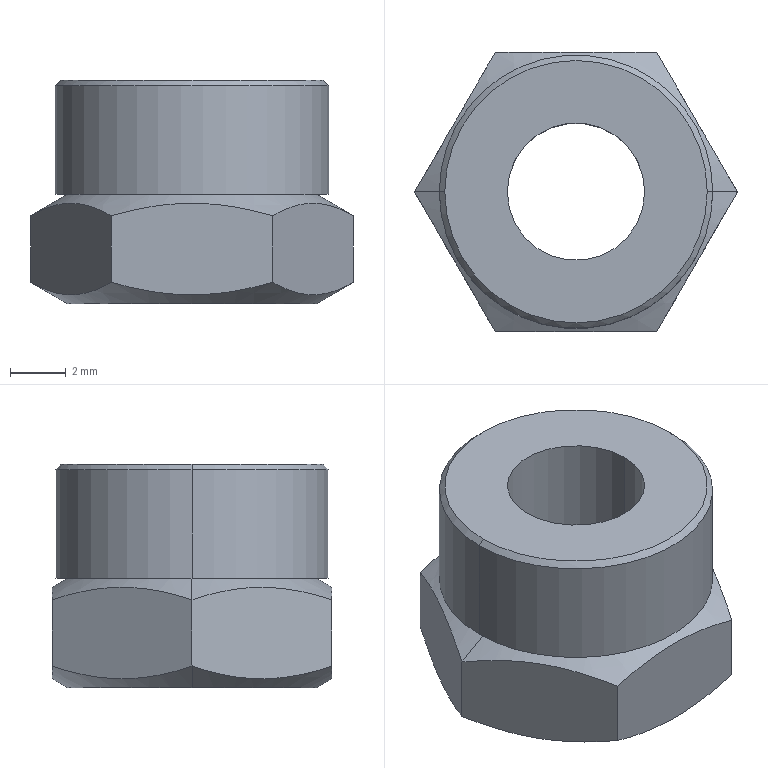Part | SolidWorks | features RevCut 3, Boss 1, Chamfer 1, Extrusion 1, LPattern 1 | 1 solid | 21 faces | box 11.547 x 10 x 8 mm | volume 473.326 mm3 | plane 9 | cone 8 | cylinder 4 | commonest cylinder face diameters 4.917 x2 9.78 x2
STEP:
#1=CARTESIAN_POINT('',(4.694,0.,4.08));
#2=VERTEX_POINT('',#1);
#3=CARTESIAN_POINT('',(-4.694,0.,4.08));
#4=VERTEX_POINT('',#3);
#5=CARTESIAN_POINT('',(0.,0.,4.08));
#6=DIRECTION('',(0.,0.,1.));
#7=DIRECTION('',(1.,0.,0.));
#8=AXIS2_PLACEMENT_3D('',#5,#6,#7);
#9=CIRCLE('',#8,4.694);
#10=EDGE_CURVE('',#2,#4,#9,.T.);
#11=ORIENTED_EDGE('',*,*,#10,.F.);
#12=CARTESIAN_POINT('',(4.89,0.,3.884));
#13=VERTEX_POINT('',#12);
#14=CARTESIAN_POINT('',(4.694,0.,4.08));
#15=DIRECTION('',(0.7071,0.,-0.7071));
#16=VECTOR('',#15,1000.);
#17=LINE('',#14,#16);
#18=EDGE_CURVE('',#2,#13,#17,.T.);
#19=ORIENTED_EDGE('',*,*,#18,.T.);
#20=CARTESIAN_POINT('',(-4.89,0.,3.884));
#21=VERTEX_POINT('',#20);
#22=CARTESIAN_POINT('',(0.,0.,3.884));
#23=DIRECTION('',(0.,0.,-1.));
#24=DIRECTION('',(1.,0.,0.));
#25=AXIS2_PLACEMENT_3D('',#22,#23,#24);
#26=CIRCLE('',#25,4.89);
#27=EDGE_CURVE('',#21,#13,#26,.T.);
#28=ORIENTED_EDGE('',*,*,#27,.F.);
#29=CARTESIAN_POINT('',(-4.694,0.,4.08));
#30=DIRECTION('',(-0.7071,0.,-0.7071));
#31=VECTOR('',#30,1000.);
#32=LINE('',#29,#31);
#33=EDGE_CURVE('',#4,#21,#32,.T.);
#34=ORIENTED_EDGE('',*,*,#33,.F.);
#35=EDGE_LOOP('',(#11,#19,#28,#34));
#36=FACE_OUTER_BOUND('',#35,.T.);
#37=CARTESIAN_POINT('',(0.,0.,4.08));
#38=DIRECTION('',(0.,0.,-1.));
#39=DIRECTION('',(-1.,0.,0.));
#40=AXIS2_PLACEMENT_3D('',#37,#38,#39);
#41=CONICAL_SURFACE('',#40,4.694,0.7854);
#42=ADVANCED_FACE('',(#36),#41,.T.);
#43=CARTESIAN_POINT('',(2.458,0.,-3.004));
#44=VERTEX_POINT('',#43);
#45=CARTESIAN_POINT('',(-2.458,0.,-3.004));
#46=VERTEX_POINT('',#45);
#47=CARTESIAN_POINT('',(0.,0.,-3.004));
#48=DIRECTION('',(0.,0.,-1.));
#49=DIRECTION('',(-1.,0.,0.));
#50=AXIS2_PLACEMENT_3D('',#47,#48,#49);
#51=CIRCLE('',#50,2.458);
#52=EDGE_CURVE('',#44,#46,#51,.T.);
#53=ORIENTED_EDGE('',*,*,#52,.F.);
#54=CARTESIAN_POINT('',(3.375,0.,-3.92));
#55=VERTEX_POINT('',#54);
#56=CARTESIAN_POINT('',(2.458,0.,-3.004));
#57=DIRECTION('',(0.7071,0.,-0.7071));
#58=VECTOR('',#57,1000.);
#59=LINE('',#56,#58);
#60=EDGE_CURVE('',#44,#55,#59,.T.);
#61=ORIENTED_EDGE('',*,*,#60,.T.);
#62=CARTESIAN_POINT('',(-3.375,0.,-3.92));
#63=VERTEX_POINT('',#62);
#64=CARTESIAN_POINT('',(0.,0.,-3.92));
#65=DIRECTION('',(0.,0.,-1.));
#66=DIRECTION('',(-1.,0.,0.));
#67=AXIS2_PLACEMENT_3D('',#64,#65,#66);
#68=CIRCLE('',#67,3.375);
#69=EDGE_CURVE('',#55,#63,#68,.T.);
#70=ORIENTED_EDGE('',*,*,#69,.T.);
#71=CARTESIAN_POINT('',(-2.458,0.,-3.004));
#72=DIRECTION('',(-0.7071,0.,-0.7071));
#73=VECTOR('',#72,1000.);
#74=LINE('',#71,#73);
#75=EDGE_CURVE('',#46,#63,#74,.T.);
#76=ORIENTED_EDGE('',*,*,#75,.F.);
#77=EDGE_LOOP('',(#53,#61,#70,#76));
#78=FACE_OUTER_BOUND('',#77,.T.);
#79=CARTESIAN_POINT('',(0.,0.,-3.004));
#80=DIRECTION('',(0.,0.,-1.));
#81=DIRECTION('',(-1.,0.,0.));
#82=AXIS2_PLACEMENT_3D('',#79,#80,#81);
#83=CONICAL_SURFACE('',#82,2.458,0.7854);
#84=ADVANCED_FACE('',(#78),#83,.F.);
#85=ORIENTED_EDGE('',*,*,#27,.T.);
#86=CARTESIAN_POINT('',(4.89,0.,0.));
#87=VERTEX_POINT('',#86);
#88=CARTESIAN_POINT('',(4.89,0.,25.911));
#89=DIRECTION('',(0.,0.,-1.));
#90=VECTOR('',#89,1000.);
#91=LINE('',#88,#90);
#92=EDGE_CURVE('',#13,#87,#91,.T.);
#93=ORIENTED_EDGE('',*,*,#92,.T.);
#94=CARTESIAN_POINT('',(-4.89,0.,0.));
#95=VERTEX_POINT('',#94);
#96=CARTESIAN_POINT('',(0.,0.,0.));
#97=DIRECTION('',(0.,0.,1.));
#98=DIRECTION('',(1.,0.,0.));
#99=AXIS2_PLACEMENT_3D('',#96,#97,#98);
#100=CIRCLE('',#99,4.89);
#101=EDGE_CURVE('',#87,#95,#100,.T.);
#102=ORIENTED_EDGE('',*,*,#101,.T.);
#103=CARTESIAN_POINT('',(-4.89,0.,25.911));
#104=DIRECTION('',(0.,0.,-1.));
#105=VECTOR('',#104,1000.);
#106=LINE('',#103,#105);
#107=EDGE_CURVE('',#21,#95,#106,.T.);
#108=ORIENTED_EDGE('',*,*,#107,.F.);
#109=EDGE_LOOP('',(#85,#93,#102,#108));
#110=FACE_OUTER_BOUND('',#109,.T.);
#111=CARTESIAN_POINT('',(0.,0.,25.911));
#112=DIRECTION('',(0.,0.,-1.));
#113=DIRECTION('',(-1.,0.,0.));
#114=AXIS2_PLACEMENT_3D('',#111,#112,#113);
#115=CYLINDRICAL_SURFACE('',#114,4.89);
#116=ADVANCED_FACE('',(#110),#115,.T.);
#117=CARTESIAN_POINT('',(-4.44,0.,0.));
#118=VERTEX_POINT('',#117);
#119=CARTESIAN_POINT('',(4.44,0.,0.));
#120=VERTEX_POINT('',#119);
#121=CARTESIAN_POINT('',(0.,0.,0.));
#122=DIRECTION('',(0.,0.,-1.));
#123=DIRECTION('',(1.,0.,0.));
#124=AXIS2_PLACEMENT_3D('',#121,#122,#123);
#125=CIRCLE('',#124,4.44);
#126=EDGE_CURVE('',#118,#120,#125,.T.);
#127=ORIENTED_EDGE('',*,*,#126,.T.);
#128=CARTESIAN_POINT('',(5.774,0.,-0.7699));
#129=VERTEX_POINT('',#128);
#130=CARTESIAN_POINT('',(5.774,0.,-0.7699));
#131=DIRECTION('',(0.866,0.,-0.5));
#132=VECTOR('',#131,1000.);
#133=LINE('',#130,#132);
#134=EDGE_CURVE('',#120,#129,#133,.T.);
#135=ORIENTED_EDGE('',*,*,#134,.T.);
#136=CARTESIAN_POINT('',(2.887,5.,-0.7699));
#137=VERTEX_POINT('',#136);
#138=CARTESIAN_POINT('',(2.887,5.,-0.7699));
#139=CARTESIAN_POINT('',(3.358,4.184,-0.4978));
#140=CARTESIAN_POINT('',(3.837,3.355,-0.3239));
#141=CARTESIAN_POINT('',(4.45,2.292,-0.3232));
#142=CARTESIAN_POINT('',(4.573,2.079,-0.3336));
#143=CARTESIAN_POINT('',(4.817,1.656,-0.3743));
#144=CARTESIAN_POINT('',(4.938,1.446,-0.4045));
#145=CARTESIAN_POINT('',(5.3,0.8208,-0.5212));
#146=CARTESIAN_POINT('',(5.538,0.4087,-0.6337));
#147=CARTESIAN_POINT('',(5.774,0.,-0.7699));
#148=B_SPLINE_CURVE_WITH_KNOTS('',3,(#138,#139,#140,#141,#142,#143,#144,#145,#146,#147),.UNSPECIFIED.,.F.,.F.,(4,2,2,2,4),(0.000000238,0.002916,0.003645,0.004373,0.005831),.UNSPECIFIED.);
#149=EDGE_CURVE('',#137,#129,#148,.T.);
#150=ORIENTED_EDGE('',*,*,#149,.F.);
#151=CARTESIAN_POINT('',(-2.887,5.,-0.7699));
#152=VERTEX_POINT('',#151);
#153=CARTESIAN_POINT('',(-2.887,5.,-0.7699));
#154=CARTESIAN_POINT('',(-2.417,5.,-0.6344));
#155=CARTESIAN_POINT('',(-1.936,5.,-0.5206));
#156=CARTESIAN_POINT('',(-0.9718,5.,-0.3652));
#157=CARTESIAN_POINT('',(-0.487,5.,-0.3233));
#158=CARTESIAN_POINT('',(0.4886,5.,-0.3234));
#159=CARTESIAN_POINT('',(0.9831,5.,-0.3664));
#160=CARTESIAN_POINT('',(1.947,5.,-0.523));
#161=CARTESIAN_POINT('',(2.42,5.,-0.6352));
#162=CARTESIAN_POINT('',(2.887,5.,-0.7699));
#163=B_SPLINE_CURVE_WITH_KNOTS('',3,(#153,#154,#155,#156,#157,#158,#159,#160,#161,#162),.UNSPECIFIED.,.F.,.F.,(4,2,2,2,4),(0.005101,0.006561,0.008021,0.009482,0.01094),.UNSPECIFIED.);
#164=EDGE_CURVE('',#152,#137,#163,.T.);
#165=ORIENTED_EDGE('',*,*,#164,.F.);
#166=CARTESIAN_POINT('',(-5.774,0.,-0.7699));
#167=VERTEX_POINT('',#166);
#168=CARTESIAN_POINT('',(-5.774,0.,-0.7699));
#169=CARTESIAN_POINT('',(-5.302,0.8164,-0.4978));
#170=CARTESIAN_POINT('',(-4.824,1.645,-0.3239));
#171=CARTESIAN_POINT('',(-4.21,2.708,-0.3232));
#172=CARTESIAN_POINT('',(-4.087,2.921,-0.3336));
#173=CARTESIAN_POINT('',(-3.843,3.344,-0.3743));
#174=CARTESIAN_POINT('',(-3.722,3.554,-0.4045));
#175=CARTESIAN_POINT('',(-3.361,4.179,-0.5212));
#176=CARTESIAN_POINT('',(-3.123,4.591,-0.6337));
#177=CARTESIAN_POINT('',(-2.887,5.,-0.7699));
#178=B_SPLINE_CURVE_WITH_KNOTS('',3,(#168,#169,#170,#171,#172,#173,#174,#175,#176,#177),.UNSPECIFIED.,.F.,.F.,(4,2,2,2,4),(0.000000238,0.002916,0.003645,0.004373,0.005831),.UNSPECIFIED.);
#179=EDGE_CURVE('',#167,#152,#178,.T.);
#180=ORIENTED_EDGE('',*,*,#179,.F.);
#181=CARTESIAN_POINT('',(-5.774,0.,-0.7699));
#182=DIRECTION('',(-0.866,0.,-0.5));
#183=VECTOR('',#182,1000.);
#184=LINE('',#181,#183);
#185=EDGE_CURVE('',#118,#167,#184,.T.);
#186=ORIENTED_EDGE('',*,*,#185,.F.);
#187=EDGE_LOOP('',(#127,#135,#150,#165,#180,#186));
#188=FACE_OUTER_BOUND('',#187,.T.);
#189=CARTESIAN_POINT('',(0.,0.,-0.7699));
#190=DIRECTION('',(0.,0.,-1.));
#191=DIRECTION('',(-1.,0.,0.));
#192=AXIS2_PLACEMENT_3D('',#189,#190,#191);
#193=CONICAL_SURFACE('',#192,5.774,1.047);
#194=ADVANCED_FACE('',(#188),#193,.T.);
#195=CARTESIAN_POINT('',(-4.44,0.,-3.92));
#196=VERTEX_POINT('',#195);
#197=CARTESIAN_POINT('',(4.44,0.,-3.92));
#198=VERTEX_POINT('',#197);
#199=CARTESIAN_POINT('',(0.,0.,-3.92));
#200=DIRECTION('',(0.,0.,-1.));
#201=DIRECTION('',(-1.,0.,0.));
#202=AXIS2_PLACEMENT_3D('',#199,#200,#201);
#203=CIRCLE('',#202,4.44);
#204=EDGE_CURVE('',#196,#198,#203,.T.);
#205=ORIENTED_EDGE('',*,*,#204,.F.);
#206=CARTESIAN_POINT('',(-5.774,0.,-3.15));
#207=VERTEX_POINT('',#206);
#208=CARTESIAN_POINT('',(-4.44,0.,-3.92));
#209=DIRECTION('',(-0.866,0.,0.5));
#210=VECTOR('',#209,1000.);
#211=LINE('',#208,#210);
#212=EDGE_CURVE('',#196,#207,#211,.T.);
#213=ORIENTED_EDGE('',*,*,#212,.T.);
#214=CARTESIAN_POINT('',(-2.887,5.,-3.15));
#215=VERTEX_POINT('',#214);
#216=CARTESIAN_POINT('',(-2.887,5.,-3.15));
#217=CARTESIAN_POINT('',(-3.358,4.184,-3.422));
#218=CARTESIAN_POINT('',(-3.837,3.355,-3.596));
#219=CARTESIAN_POINT('',(-4.45,2.292,-3.597));
#220=CARTESIAN_POINT('',(-4.573,2.079,-3.586));
#221=CARTESIAN_POINT('',(-4.817,1.656,-3.546));
#222=CARTESIAN_POINT('',(-4.938,1.446,-3.515));
#223=CARTESIAN_POINT('',(-5.3,0.8208,-3.399));
#224=CARTESIAN_POINT('',(-5.538,0.4087,-3.286));
#225=CARTESIAN_POINT('',(-5.774,0.,-3.15));
#226=B_SPLINE_CURVE_WITH_KNOTS('',3,(#216,#217,#218,#219,#220,#221,#222,#223,#224,#225),.UNSPECIFIED.,.F.,.F.,(4,2,2,2,4),(0.000000238,0.002916,0.003645,0.004373,0.005831),.UNSPECIFIED.);
#227=EDGE_CURVE('',#215,#207,#226,.T.);
#228=ORIENTED_EDGE('',*,*,#227,.F.);
#229=CARTESIAN_POINT('',(2.887,5.,-3.15));
#230=VERTEX_POINT('',#229);
#231=CARTESIAN_POINT('',(2.887,5.,-3.15));
#232=CARTESIAN_POINT('',(2.42,5.,-3.285));
#233=CARTESIAN_POINT('',(1.947,5.,-3.397));
#234=CARTESIAN_POINT('',(0.9831,5.,-3.554));
#235=CARTESIAN_POINT('',(0.4886,5.,-3.597));
#236=CARTESIAN_POINT('',(-0.487,5.,-3.597));
#237=CARTESIAN_POINT('',(-0.9718,5.,-3.555));
#238=CARTESIAN_POINT('',(-1.936,5.,-3.399));
#239=CARTESIAN_POINT('',(-2.417,5.,-3.286));
#240=CARTESIAN_POINT('',(-2.887,5.,-3.15));
#241=B_SPLINE_CURVE_WITH_KNOTS('',3,(#231,#232,#233,#234,#235,#236,#237,#238,#239,#240),.UNSPECIFIED.,.F.,.F.,(4,2,2,2,4),(0.01286,0.01432,0.01578,0.01724,0.01871),.UNSPECIFIED.);
#242=EDGE_CURVE('',#230,#215,#241,.T.);
#243=ORIENTED_EDGE('',*,*,#242,.F.);
#244=CARTESIAN_POINT('',(5.774,0.,-3.15));
#245=VERTEX_POINT('',#244);
#246=CARTESIAN_POINT('',(5.774,0.,-3.15));
#247=CARTESIAN_POINT('',(5.302,0.8164,-3.422));
#248=CARTESIAN_POINT('',(4.824,1.645,-3.596));
#249=CARTESIAN_POINT('',(4.21,2.708,-3.597));
#250=CARTESIAN_POINT('',(4.087,2.921,-3.586));
#251=CARTESIAN_POINT('',(3.843,3.344,-3.546));
#252=CARTESIAN_POINT('',(3.722,3.554,-3.515));
#253=CARTESIAN_POINT('',(3.361,4.179,-3.399));
#254=CARTESIAN_POINT('',(3.123,4.591,-3.286));
#255=CARTESIAN_POINT('',(2.887,5.,-3.15));
#256=B_SPLINE_CURVE_WITH_KNOTS('',3,(#246,#247,#248,#249,#250,#251,#252,#253,#254,#255),.UNSPECIFIED.,.F.,.F.,(4,2,2,2,4),(0.000000238,0.002916,0.003645,0.004373,0.005831),.UNSPECIFIED.);
#257=EDGE_CURVE('',#245,#230,#256,.T.);
#258=ORIENTED_EDGE('',*,*,#257,.F.);
#259=CARTESIAN_POINT('',(4.44,0.,-3.92));
#260=DIRECTION('',(0.866,0.,0.5));
#261=VECTOR('',#260,1000.);
#262=LINE('',#259,#261);
#263=EDGE_CURVE('',#198,#245,#262,.T.);
#264=ORIENTED_EDGE('',*,*,#263,.F.);
#265=EDGE_LOOP('',(#205,#213,#228,#243,#258,#264));
#266=FACE_OUTER_BOUND('',#265,.T.);
#267=CARTESIAN_POINT('',(0.,0.,-3.92));
#268=DIRECTION('',(0.,0.,1.));
#269=DIRECTION('',(1.,0.,0.));
#270=AXIS2_PLACEMENT_3D('',#267,#268,#269);
#271=CONICAL_SURFACE('',#270,4.44,1.047);
#272=ADVANCED_FACE('',(#266),#271,.T.);
#273=ORIENTED_EDGE('',*,*,#52,.T.);
#274=CARTESIAN_POINT('',(-2.458,0.,4.08));
#275=VERTEX_POINT('',#274);
#276=CARTESIAN_POINT('',(-2.458,0.,-3.92));
#277=DIRECTION('',(0.,0.,1.));
#278=VECTOR('',#277,1000.);
#279=LINE('',#276,#278);
#280=EDGE_CURVE('',#46,#275,#279,.T.);
#281=ORIENTED_EDGE('',*,*,#280,.T.);
#282=CARTESIAN_POINT('',(2.458,0.,4.08));
#283=VERTEX_POINT('',#282);
#284=CARTESIAN_POINT('',(0.,0.,4.08));
#285=DIRECTION('',(0.,0.,1.));
#286=DIRECTION('',(1.,0.,0.));
#287=AXIS2_PLACEMENT_3D('',#284,#285,#286);
#288=CIRCLE('',#287,2.458);
#289=EDGE_CURVE('',#275,#283,#288,.T.);
#290=ORIENTED_EDGE('',*,*,#289,.T.);
#291=CARTESIAN_POINT('',(2.458,0.,-3.92));
#292=DIRECTION('',(0.,0.,1.));
#293=VECTOR('',#292,1000.);
#294=LINE('',#291,#293);
#295=EDGE_CURVE('',#44,#283,#294,.T.);
#296=ORIENTED_EDGE('',*,*,#295,.F.);
#297=EDGE_LOOP('',(#273,#281,#290,#296));
#298=FACE_OUTER_BOUND('',#297,.T.);
#299=CARTESIAN_POINT('',(0.,0.,-3.92));
#300=DIRECTION('',(0.,0.,1.));
#301=DIRECTION('',(1.,0.,0.));
#302=AXIS2_PLACEMENT_3D('',#299,#300,#301);
#303=CYLINDRICAL_SURFACE('',#302,2.458);
#304=ADVANCED_FACE('',(#298),#303,.F.);
#305=CARTESIAN_POINT('',(0.,0.,-3.92));
#306=DIRECTION('',(0.,0.,-1.));
#307=DIRECTION('',(-1.,0.,0.));
#308=AXIS2_PLACEMENT_3D('',#305,#306,#307);
#309=CIRCLE('',#308,4.44);
#310=EDGE_CURVE('',#198,#196,#309,.T.);
#311=ORIENTED_EDGE('',*,*,#310,.T.);
#312=ORIENTED_EDGE('',*,*,#204,.T.);
#313=EDGE_LOOP('',(#311,#312));
#314=FACE_OUTER_BOUND('',#313,.T.);
#315=CARTESIAN_POINT('',(0.,0.,-3.92));
#316=DIRECTION('',(0.,0.,-1.));
#317=DIRECTION('',(-1.,0.,0.));
#318=AXIS2_PLACEMENT_3D('',#315,#316,#317);
#319=CIRCLE('',#318,3.375);
#320=EDGE_CURVE('',#63,#55,#319,.T.);
#321=ORIENTED_EDGE('',*,*,#320,.F.);
#322=ORIENTED_EDGE('',*,*,#69,.F.);
#323=EDGE_LOOP('',(#321,#322));
#324=FACE_BOUND('',#323,.T.);
#325=CARTESIAN_POINT('',(2.887,-5.,-3.92));
#326=DIRECTION('',(0.,0.,1.));
#327=DIRECTION('',(1.,0.,0.));
#328=AXIS2_PLACEMENT_3D('',#325,#326,#327);
#329=PLANE('',#328);
#330=ADVANCED_FACE('',(#314,#324),#329,.F.);
#331=ORIENTED_EDGE('',*,*,#280,.F.);
#332=CARTESIAN_POINT('',(0.,0.,-3.004));
#333=DIRECTION('',(0.,0.,-1.));
#334=DIRECTION('',(-1.,0.,0.));
#335=AXIS2_PLACEMENT_3D('',#332,#333,#334);
#336=CIRCLE('',#335,2.458);
#337=EDGE_CURVE('',#46,#44,#336,.T.);
#338=ORIENTED_EDGE('',*,*,#337,.T.);
#339=ORIENTED_EDGE('',*,*,#295,.T.);
#340=CARTESIAN_POINT('',(0.,0.,4.08));
#341=DIRECTION('',(0.,0.,1.));
#342=DIRECTION('',(1.,0.,0.));
#343=AXIS2_PLACEMENT_3D('',#340,#341,#342);
#344=CIRCLE('',#343,2.458);
#345=EDGE_CURVE('',#283,#275,#344,.T.);
#346=ORIENTED_EDGE('',*,*,#345,.T.);
#347=EDGE_LOOP('',(#331,#338,#339,#346));
#348=FACE_OUTER_BOUND('',#347,.T.);
#349=CARTESIAN_POINT('',(0.,0.,-3.92));
#350=DIRECTION('',(0.,0.,1.));
#351=DIRECTION('',(1.,0.,0.));
#352=AXIS2_PLACEMENT_3D('',#349,#350,#351);
#353=CYLINDRICAL_SURFACE('',#352,2.458);
#354=ADVANCED_FACE('',(#348),#353,.F.);
#355=CARTESIAN_POINT('',(2.887,-5.,-3.15));
#356=VERTEX_POINT('',#355);
#357=CARTESIAN_POINT('',(2.887,-5.,-0.7699));
#358=VERTEX_POINT('',#357);
#359=CARTESIAN_POINT('',(2.887,-5.,-3.92));
#360=DIRECTION('',(0.,0.,1.));
#361=VECTOR('',#360,1000.);
#362=LINE('',#359,#361);
#363=EDGE_CURVE('',#356,#358,#362,.T.);
#364=ORIENTED_EDGE('',*,*,#363,.T.);
#365=CARTESIAN_POINT('',(-2.887,-5.,-0.7699));
#366=VERTEX_POINT('',#365);
#367=CARTESIAN_POINT('',(2.887,-5.,-0.7699));
#368=CARTESIAN_POINT('',(2.42,-5.,-0.6352));
#369=CARTESIAN_POINT('',(1.947,-5.,-0.523));
#370=CARTESIAN_POINT('',(0.9831,-5.,-0.3664));
#371=CARTESIAN_POINT('',(0.4886,-5.,-0.3234));
#372=CARTESIAN_POINT('',(-0.487,-5.,-0.3233));
#373=CARTESIAN_POINT('',(-0.9718,-5.,-0.3652));
#374=CARTESIAN_POINT('',(-1.936,-5.,-0.5206));
#375=CARTESIAN_POINT('',(-2.417,-5.,-0.6344));
#376=CARTESIAN_POINT('',(-2.887,-5.,-0.7699));
#377=B_SPLINE_CURVE_WITH_KNOTS('',3,(#367,#368,#369,#370,#371,#372,#373,#374,#375,#376),.UNSPECIFIED.,.F.,.F.,(4,2,2,2,4),(0.01286,0.01432,0.01578,0.01724,0.01871),.UNSPECIFIED.);
#378=EDGE_CURVE('',#358,#366,#377,.T.);
#379=ORIENTED_EDGE('',*,*,#378,.T.);
#380=CARTESIAN_POINT('',(-2.887,-5.,-3.15));
#381=VERTEX_POINT('',#380);
#382=CARTESIAN_POINT('',(-2.887,-5.,-3.92));
#383=DIRECTION('',(0.,0.,1.));
#384=VECTOR('',#383,1000.);
#385=LINE('',#382,#384);
#386=EDGE_CURVE('',#381,#366,#385,.T.);
#387=ORIENTED_EDGE('',*,*,#386,.F.);
#388=CARTESIAN_POINT('',(-2.887,-5.,-3.15));
#389=CARTESIAN_POINT('',(-2.417,-5.,-3.286));
#390=CARTESIAN_POINT('',(-1.936,-5.,-3.399));
#391=CARTESIAN_POINT('',(-0.9718,-5.,-3.555));
#392=CARTESIAN_POINT('',(-0.487,-5.,-3.597));
#393=CARTESIAN_POINT('',(0.4886,-5.,-3.597));
#394=CARTESIAN_POINT('',(0.9831,-5.,-3.554));
#395=CARTESIAN_POINT('',(1.947,-5.,-3.397));
#396=CARTESIAN_POINT('',(2.42,-5.,-3.285));
#397=CARTESIAN_POINT('',(2.887,-5.,-3.15));
#398=B_SPLINE_CURVE_WITH_KNOTS('',3,(#388,#389,#390,#391,#392,#393,#394,#395,#396,#397),.UNSPECIFIED.,.F.,.F.,(4,2,2,2,4),(0.005101,0.006561,0.008021,0.009482,0.01094),.UNSPECIFIED.);
#399=EDGE_CURVE('',#381,#356,#398,.T.);
#400=ORIENTED_EDGE('',*,*,#399,.T.);
#401=EDGE_LOOP('',(#364,#379,#387,#400));
#402=FACE_OUTER_BOUND('',#401,.T.);
#403=CARTESIAN_POINT('',(-2.887,-5.,-3.92));
#404=DIRECTION('',(0.,-1.,0.));
#405=DIRECTION('',(1.,0.,0.));
#406=AXIS2_PLACEMENT_3D('',#403,#404,#405);
#407=PLANE('',#406);
#408=ADVANCED_FACE('',(#402),#407,.T.);
#409=ORIENTED_EDGE('',*,*,#386,.T.);
#410=CARTESIAN_POINT('',(-2.887,-5.,-0.7699));
#411=CARTESIAN_POINT('',(-3.358,-4.184,-0.4978));
#412=CARTESIAN_POINT('',(-3.837,-3.355,-0.3239));
#413=CARTESIAN_POINT('',(-4.45,-2.292,-0.3232));
#414=CARTESIAN_POINT('',(-4.573,-2.079,-0.3336));
#415=CARTESIAN_POINT('',(-4.817,-1.656,-0.3743));
#416=CARTESIAN_POINT('',(-4.938,-1.446,-0.4045));
#417=CARTESIAN_POINT('',(-5.3,-0.8208,-0.5212));
#418=CARTESIAN_POINT('',(-5.538,-0.4087,-0.6337));
#419=CARTESIAN_POINT('',(-5.774,0.,-0.7699));
#420=B_SPLINE_CURVE_WITH_KNOTS('',3,(#410,#411,#412,#413,#414,#415,#416,#417,#418,#419),.UNSPECIFIED.,.F.,.F.,(4,2,2,2,4),(0.000000238,0.002916,0.003645,0.004373,0.005831),.UNSPECIFIED.);
#421=EDGE_CURVE('',#366,#167,#420,.T.);
#422=ORIENTED_EDGE('',*,*,#421,.T.);
#423=CARTESIAN_POINT('',(-5.774,0.,-3.92));
#424=DIRECTION('',(0.,0.,1.));
#425=VECTOR('',#424,1000.);
#426=LINE('',#423,#425);
#427=EDGE_CURVE('',#207,#167,#426,.T.);
#428=ORIENTED_EDGE('',*,*,#427,.F.);
#429=CARTESIAN_POINT('',(-5.774,0.,-3.15));
#430=CARTESIAN_POINT('',(-5.302,-0.8164,-3.422));
#431=CARTESIAN_POINT('',(-4.824,-1.645,-3.596));
#432=CARTESIAN_POINT('',(-4.21,-2.708,-3.597));
#433=CARTESIAN_POINT('',(-4.087,-2.921,-3.586));
#434=CARTESIAN_POINT('',(-3.843,-3.344,-3.546));
#435=CARTESIAN_POINT('',(-3.722,-3.554,-3.515));
#436=CARTESIAN_POINT('',(-3.361,-4.179,-3.399));
#437=CARTESIAN_POINT('',(-3.123,-4.591,-3.286));
#438=CARTESIAN_POINT('',(-2.887,-5.,-3.15));
#439=B_SPLINE_CURVE_WITH_KNOTS('',3,(#429,#430,#431,#432,#433,#434,#435,#436,#437,#438),.UNSPECIFIED.,.F.,.F.,(4,2,2,2,4),(0.000000238,0.002916,0.003645,0.004373,0.005831),.UNSPECIFIED.);
#440=EDGE_CURVE('',#207,#381,#439,.T.);
#441=ORIENTED_EDGE('',*,*,#440,.T.);
#442=EDGE_LOOP('',(#409,#422,#428,#441));
#443=FACE_OUTER_BOUND('',#442,.T.);
#444=CARTESIAN_POINT('',(-5.774,0.,-3.92));
#445=DIRECTION('',(-0.866,-0.5,0.));
#446=DIRECTION('',(0.5,-0.866,0.));
#447=AXIS2_PLACEMENT_3D('',#444,#445,#446);
#448=PLANE('',#447);
#449=ADVANCED_FACE('',(#443),#448,.T.);
#450=ORIENTED_EDGE('',*,*,#427,.T.);
#451=ORIENTED_EDGE('',*,*,#179,.T.);
#452=CARTESIAN_POINT('',(-2.887,5.,-3.92));
#453=DIRECTION('',(0.,0.,1.));
#454=VECTOR('',#453,1000.);
#455=LINE('',#452,#454);
#456=EDGE_CURVE('',#215,#152,#455,.T.);
#457=ORIENTED_EDGE('',*,*,#456,.F.);
#458=ORIENTED_EDGE('',*,*,#227,.T.);
#459=EDGE_LOOP('',(#450,#451,#457,#458));
#460=FACE_OUTER_BOUND('',#459,.T.);
#461=CARTESIAN_POINT('',(-2.887,5.,-3.92));
#462=DIRECTION('',(-0.866,0.5,0.));
#463=DIRECTION('',(-0.5,-0.866,0.));
#464=AXIS2_PLACEMENT_3D('',#461,#462,#463);
#465=PLANE('',#464);
#466=ADVANCED_FACE('',(#460),#465,.T.);
#467=ORIENTED_EDGE('',*,*,#456,.T.);
#468=ORIENTED_EDGE('',*,*,#164,.T.);
#469=CARTESIAN_POINT('',(2.887,5.,-3.92));
#470=DIRECTION('',(0.,0.,1.));
#471=VECTOR('',#470,1000.);
#472=LINE('',#469,#471);
#473=EDGE_CURVE('',#230,#137,#472,.T.);
#474=ORIENTED_EDGE('',*,*,#473,.F.);
#475=ORIENTED_EDGE('',*,*,#242,.T.);
#476=EDGE_LOOP('',(#467,#468,#474,#475));
#477=FACE_OUTER_BOUND('',#476,.T.);
#478=CARTESIAN_POINT('',(2.887,5.,-3.92));
#479=DIRECTION('',(0.,1.,0.));
#480=DIRECTION('',(0.,0.,1.));
#481=AXIS2_PLACEMENT_3D('',#478,#479,#480);
#482=PLANE('',#481);
#483=ADVANCED_FACE('',(#477),#482,.T.);
#484=ORIENTED_EDGE('',*,*,#473,.T.);
#485=ORIENTED_EDGE('',*,*,#149,.T.);
#486=CARTESIAN_POINT('',(5.774,0.,-3.92));
#487=DIRECTION('',(0.,0.,1.));
#488=VECTOR('',#487,1000.);
#489=LINE('',#486,#488);
#490=EDGE_CURVE('',#245,#129,#489,.T.);
#491=ORIENTED_EDGE('',*,*,#490,.F.);
#492=ORIENTED_EDGE('',*,*,#257,.T.);
#493=EDGE_LOOP('',(#484,#485,#491,#492));
#494=FACE_OUTER_BOUND('',#493,.T.);
#495=CARTESIAN_POINT('',(5.774,0.,-3.92));
#496=DIRECTION('',(0.866,0.5,0.));
#497=DIRECTION('',(-0.5,0.866,0.));
#498=AXIS2_PLACEMENT_3D('',#495,#496,#497);
#499=PLANE('',#498);
#500=ADVANCED_FACE('',(#494),#499,.T.);
#501=ORIENTED_EDGE('',*,*,#490,.T.);
#502=CARTESIAN_POINT('',(5.774,0.,-0.7699));
#503=CARTESIAN_POINT('',(5.302,-0.8164,-0.4978));
#504=CARTESIAN_POINT('',(4.824,-1.645,-0.3239));
#505=CARTESIAN_POINT('',(4.21,-2.708,-0.3232));
#506=CARTESIAN_POINT('',(4.087,-2.921,-0.3336));
#507=CARTESIAN_POINT('',(3.843,-3.344,-0.3743));
#508=CARTESIAN_POINT('',(3.722,-3.554,-0.4045));
#509=CARTESIAN_POINT('',(3.361,-4.179,-0.5212));
#510=CARTESIAN_POINT('',(3.123,-4.591,-0.6337));
#511=CARTESIAN_POINT('',(2.887,-5.,-0.7699));
#512=B_SPLINE_CURVE_WITH_KNOTS('',3,(#502,#503,#504,#505,#506,#507,#508,#509,#510,#511),.UNSPECIFIED.,.F.,.F.,(4,2,2,2,4),(0.000000238,0.002916,0.003645,0.004373,0.005831),.UNSPECIFIED.);
#513=EDGE_CURVE('',#129,#358,#512,.T.);
#514=ORIENTED_EDGE('',*,*,#513,.T.);
#515=ORIENTED_EDGE('',*,*,#363,.F.);
#516=CARTESIAN_POINT('',(2.887,-5.,-3.15));
#517=CARTESIAN_POINT('',(3.358,-4.184,-3.422));
#518=CARTESIAN_POINT('',(3.837,-3.355,-3.596));
#519=CARTESIAN_POINT('',(4.45,-2.292,-3.597));
#520=CARTESIAN_POINT('',(4.573,-2.079,-3.586));
#521=CARTESIAN_POINT('',(4.817,-1.656,-3.546));
#522=CARTESIAN_POINT('',(4.938,-1.446,-3.515));
#523=CARTESIAN_POINT('',(5.3,-0.8208,-3.399));
#524=CARTESIAN_POINT('',(5.538,-0.4087,-3.286));
#525=CARTESIAN_POINT('',(5.774,0.,-3.15));
#526=B_SPLINE_CURVE_WITH_KNOTS('',3,(#516,#517,#518,#519,#520,#521,#522,#523,#524,#525),.UNSPECIFIED.,.F.,.F.,(4,2,2,2,4),(0.000000238,0.002916,0.003645,0.004373,0.005831),.UNSPECIFIED.);
#527=EDGE_CURVE('',#356,#245,#526,.T.);
#528=ORIENTED_EDGE('',*,*,#527,.T.);
#529=EDGE_LOOP('',(#501,#514,#515,#528));
#530=FACE_OUTER_BOUND('',#529,.T.);
#531=CARTESIAN_POINT('',(2.887,-5.,-3.92));
#532=DIRECTION('',(0.866,-0.5,0.));
#533=DIRECTION('',(0.5,0.866,0.));
#534=AXIS2_PLACEMENT_3D('',#531,#532,#533);
#535=PLANE('',#534);
#536=ADVANCED_FACE('',(#530),#535,.T.);
#537=ORIENTED_EDGE('',*,*,#212,.F.);
#538=ORIENTED_EDGE('',*,*,#310,.F.);
#539=ORIENTED_EDGE('',*,*,#263,.T.);
#540=ORIENTED_EDGE('',*,*,#527,.F.);
#541=ORIENTED_EDGE('',*,*,#399,.F.);
#542=ORIENTED_EDGE('',*,*,#440,.F.);
#543=EDGE_LOOP('',(#537,#538,#539,#540,#541,#542));
#544=FACE_OUTER_BOUND('',#543,.T.);
#545=CARTESIAN_POINT('',(0.,0.,-3.92));
#546=DIRECTION('',(0.,0.,1.));
#547=DIRECTION('',(1.,0.,0.));
#548=AXIS2_PLACEMENT_3D('',#545,#546,#547);
#549=CONICAL_SURFACE('',#548,4.44,1.047);
#550=ADVANCED_FACE('',(#544),#549,.T.);
#551=ORIENTED_EDGE('',*,*,#134,.F.);
#552=CARTESIAN_POINT('',(0.,0.,0.));
#553=DIRECTION('',(0.,0.,-1.));
#554=DIRECTION('',(1.,0.,0.));
#555=AXIS2_PLACEMENT_3D('',#552,#553,#554);
#556=CIRCLE('',#555,4.44);
#557=EDGE_CURVE('',#120,#118,#556,.T.);
#558=ORIENTED_EDGE('',*,*,#557,.T.);
#559=ORIENTED_EDGE('',*,*,#185,.T.);
#560=ORIENTED_EDGE('',*,*,#421,.F.);
#561=ORIENTED_EDGE('',*,*,#378,.F.);
#562=ORIENTED_EDGE('',*,*,#513,.F.);
#563=EDGE_LOOP('',(#551,#558,#559,#560,#561,#562));
#564=FACE_OUTER_BOUND('',#563,.T.);
#565=CARTESIAN_POINT('',(0.,0.,-0.7699));
#566=DIRECTION('',(0.,0.,-1.));
#567=DIRECTION('',(-1.,0.,0.));
#568=AXIS2_PLACEMENT_3D('',#565,#566,#567);
#569=CONICAL_SURFACE('',#568,5.774,1.047);
#570=ADVANCED_FACE('',(#564),#569,.T.);
#571=ORIENTED_EDGE('',*,*,#92,.F.);
#572=CARTESIAN_POINT('',(0.,0.,3.884));
#573=DIRECTION('',(0.,0.,-1.));
#574=DIRECTION('',(1.,0.,0.));
#575=AXIS2_PLACEMENT_3D('',#572,#573,#574);
#576=CIRCLE('',#575,4.89);
#577=EDGE_CURVE('',#13,#21,#576,.T.);
#578=ORIENTED_EDGE('',*,*,#577,.T.);
#579=ORIENTED_EDGE('',*,*,#107,.T.);
#580=CARTESIAN_POINT('',(0.,0.,0.));
#581=DIRECTION('',(0.,0.,1.));
#582=DIRECTION('',(1.,0.,0.));
#583=AXIS2_PLACEMENT_3D('',#580,#581,#582);
#584=CIRCLE('',#583,4.89);
#585=EDGE_CURVE('',#95,#87,#584,.T.);
#586=ORIENTED_EDGE('',*,*,#585,.T.);
#587=EDGE_LOOP('',(#571,#578,#579,#586));
#588=FACE_OUTER_BOUND('',#587,.T.);
#589=CARTESIAN_POINT('',(0.,0.,25.911));
#590=DIRECTION('',(0.,0.,-1.));
#591=DIRECTION('',(-1.,0.,0.));
#592=AXIS2_PLACEMENT_3D('',#589,#590,#591);
#593=CYLINDRICAL_SURFACE('',#592,4.89);
#594=ADVANCED_FACE('',(#588),#593,.T.);
#595=ORIENTED_EDGE('',*,*,#126,.F.);
#596=ORIENTED_EDGE('',*,*,#557,.F.);
#597=EDGE_LOOP('',(#595,#596));
#598=FACE_BOUND('',#597,.T.);
#599=ORIENTED_EDGE('',*,*,#585,.F.);
#600=ORIENTED_EDGE('',*,*,#101,.F.);
#601=EDGE_LOOP('',(#599,#600));
#602=FACE_OUTER_BOUND('',#601,.T.);
#603=CARTESIAN_POINT('',(0.,0.,0.));
#604=DIRECTION('',(0.,0.,1.));
#605=DIRECTION('',(1.,0.,0.));
#606=AXIS2_PLACEMENT_3D('',#603,#604,#605);
#607=PLANE('',#606);
#608=ADVANCED_FACE('',(#598,#602),#607,.F.);
#609=CARTESIAN_POINT('',(0.,0.,4.08));
#610=DIRECTION('',(0.,0.,1.));
#611=DIRECTION('',(1.,0.,0.));
#612=AXIS2_PLACEMENT_3D('',#609,#610,#611);
#613=CIRCLE('',#612,4.694);
#614=EDGE_CURVE('',#4,#2,#613,.T.);
#615=ORIENTED_EDGE('',*,*,#614,.T.);
#616=ORIENTED_EDGE('',*,*,#10,.T.);
#617=EDGE_LOOP('',(#615,#616));
#618=FACE_OUTER_BOUND('',#617,.T.);
#619=ORIENTED_EDGE('',*,*,#345,.F.);
#620=ORIENTED_EDGE('',*,*,#289,.F.);
#621=EDGE_LOOP('',(#619,#620));
#622=FACE_BOUND('',#621,.T.);
#623=CARTESIAN_POINT('',(2.887,-5.,4.08));
#624=DIRECTION('',(0.,0.,1.));
#625=DIRECTION('',(1.,0.,0.));
#626=AXIS2_PLACEMENT_3D('',#623,#624,#625);
#627=PLANE('',#626);
#628=ADVANCED_FACE('',(#618,#622),#627,.T.);
#629=ORIENTED_EDGE('',*,*,#60,.F.);
#630=ORIENTED_EDGE('',*,*,#337,.F.);
#631=ORIENTED_EDGE('',*,*,#75,.T.);
#632=ORIENTED_EDGE('',*,*,#320,.T.);
#633=EDGE_LOOP('',(#629,#630,#631,#632));
#634=FACE_OUTER_BOUND('',#633,.T.);
#635=CARTESIAN_POINT('',(0.,0.,-3.004));
#636=DIRECTION('',(0.,0.,-1.));
#637=DIRECTION('',(-1.,0.,0.));
#638=AXIS2_PLACEMENT_3D('',#635,#636,#637);
#639=CONICAL_SURFACE('',#638,2.458,0.7854);
#640=ADVANCED_FACE('',(#634),#639,.F.);
#641=ORIENTED_EDGE('',*,*,#18,.F.);
#642=ORIENTED_EDGE('',*,*,#614,.F.);
#643=ORIENTED_EDGE('',*,*,#33,.T.);
#644=ORIENTED_EDGE('',*,*,#577,.F.);
#645=EDGE_LOOP('',(#641,#642,#643,#644));
#646=FACE_OUTER_BOUND('',#645,.T.);
#647=CARTESIAN_POINT('',(0.,0.,4.08));
#648=DIRECTION('',(0.,0.,-1.));
#649=DIRECTION('',(-1.,0.,0.));
#650=AXIS2_PLACEMENT_3D('',#647,#648,#649);
#651=CONICAL_SURFACE('',#650,4.694,0.7854);
#652=ADVANCED_FACE('',(#646),#651,.T.);
#653=CLOSED_SHELL('',(#42,#84,#116,#194,#272,#304,#330,#354,#408,#449,#466,#483,#500,#536,#550,#570,#594,#608,#628,#640,#652));
#654=MANIFOLD_SOLID_BREP('',#653);
#655=CARTESIAN_POINT('',(0.,0.,0.));
#656=DIRECTION('',(0.,0.,1.));
#657=DIRECTION('',(1.,0.,0.));
#658=AXIS2_PLACEMENT_3D('',#655,#656,#657);
#659=(LENGTH_UNIT()NAMED_UNIT(*)SI_UNIT(.MILLI.,.METRE.));
#660=UNCERTAINTY_MEASURE_WITH_UNIT(LENGTH_MEASURE(0.00001),#659,'','');
#661=(NAMED_UNIT(*)PLANE_ANGLE_UNIT()SI_UNIT($,.RADIAN.));
#662=(NAMED_UNIT(*)SI_UNIT($,.STERADIAN.)SOLID_ANGLE_UNIT());
#663=(GEOMETRIC_REPRESENTATION_CONTEXT(3)GLOBAL_UNCERTAINTY_ASSIGNED_CONTEXT((#660))GLOBAL_UNIT_ASSIGNED_CONTEXT((#659,#661,#662))REPRESENTATION_CONTEXT('',''));
#664=ADVANCED_BREP_SHAPE_REPRESENTATION('',(#654,#658),#663);